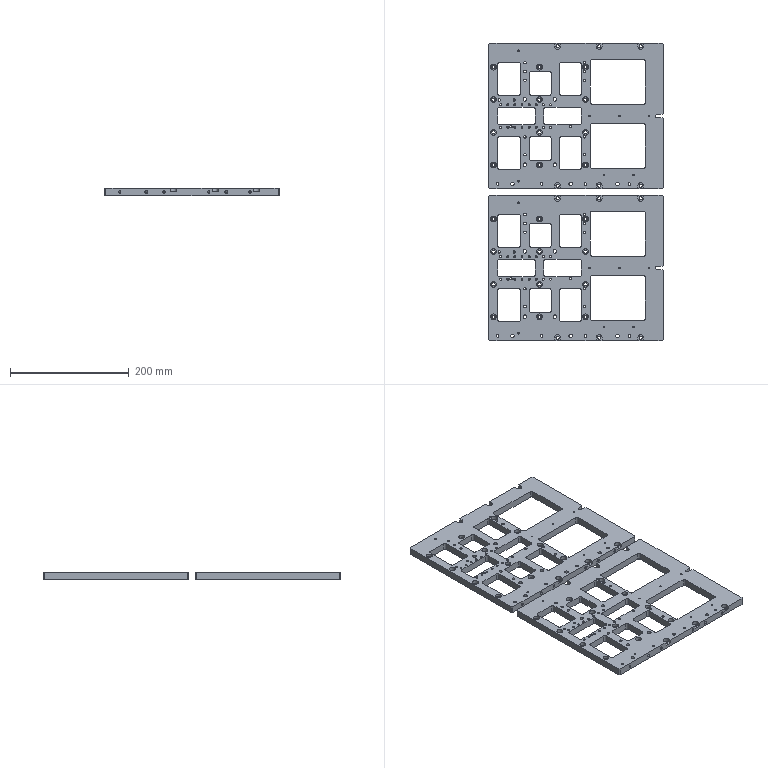Part | 2 solids | 500 faces | box 294 x 501 x 12 mm | volume 993202 mm3 | cylinder 310 | plane 170 | cone 20 | commonest cylinder face diameters 6 x96 3.3 x64 4.2 x40 5.5 x36 10 x36 4 x12